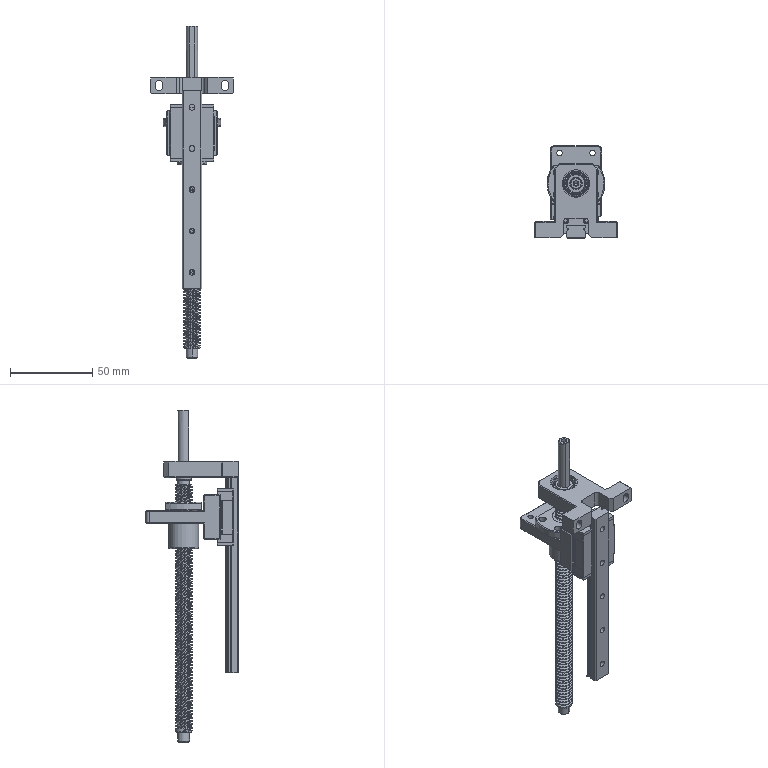Part | NX | features BREP 12 | 12 solids | 2104 faces | box 50 x 56 x 201.3 mm | volume 60246 mm3 | plane 1551 | cylinder 380 | sphere 80 | torus 47 | cone 44 | spline 2 | commonest cylinder face diameters 10 x152 0.4 x32 3.5 x18 2.571 x16 3.3 x16 7 x15